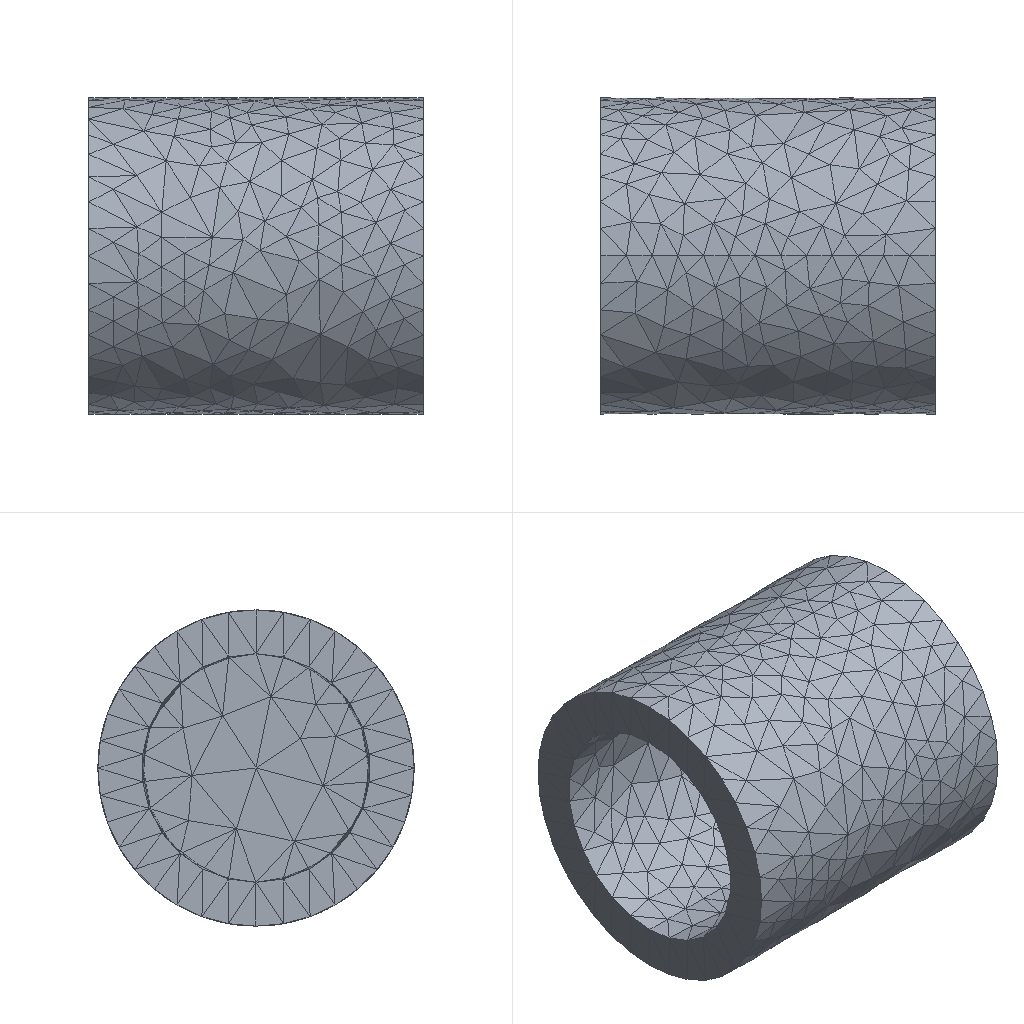Simulation study | ansys workbench
Ansys APDL input file, long lists of numbers shortened:
/batch
/config,noeldb,1     ! force off writing results to database
*get,_wallstrt,active,,time,wall
! ANSYS input file written by Workbench version 2022 R1
! File used for geometry attach:
/title,wbnew--____ (A5)
! ****** Begin Custom Load Command Snippet ******
/COM, ACT Extensions:
/COM,     LSDYNA, 2021.1
/COM,
! ****** End   Custom Load Command Snippet ******
*DIM,_wb_ProjectScratch_dir,string,248
_wb_ProjectScratch_dir(1) = ''
*DIM,_wb_SolverFiles_dir,string,248
_wb_SolverFiles_dir(1) = ''
*DIM,_wb_userfiles_dir,string,248
_wb_userfiles_dir(1) = ''
/com,--- Data in consistent NMM units. See Solving Units in the help system for more information.
/units,MPA
/nopr
/wb,file,start              !  signify a WB generated input file
/prep7
! Turn off shape checking because checks already performed inside WB mesher.
! See help system for more information.
SHPP,OFF,,NOWARN
/nolist
etcon,set             ! allow ANSYS to choose best KEYOP's for 180x elements, resets any applicable keyopt to MAPDL defaults
/com,*********** Nodes for the whole assembly ***********
nblock,3,,5894
(1i9,3e20.9e3)
        1     1.304000000E+03     0.000000000E+00     1.443258926E+02
! (5358 more lines like these left out)
-1
/wb,elem,start            !  set before creation of elements
/com,*********** Elements for Body 1 "__1-FreeParts|__-__1" ***********
et,1,187
eblock,19,solid,,2968
(19i9)
        1        1        1        1        0        0        0        0       10        0        1      310      463      855      443     2861     3860     2866     2860
! (5935 more lines like these left out)
-1
/wb,elem,end               !  done creating elements
/com,*********** Send User Defined Coordinate System(s) ***********
csys,0
toffst,273.15,  ! Temperature offset from absolute zero
/com,*********** Set Reference Temperature ***********
tref,22.
/wb,mat,start              !  starting to send materials
/com,*********** Send Materials ***********
Temperature = 'TEMP' ! Temperature
MP,DENS,1,7.85e-09,	! tonne mm^-3
MP,ALPX,1,1.2e-05,	! C^-1
MP,C,1,434000000,	! mm^2 s^-2 C^-1
MP,KXX,1,60.5,	! tonne mm s^-3 C^-1
MP,RSVX,1,0.00017,	! ohm mm
MP,EX,1,200000,	! tonne s^-2 mm^-1
MP,NUXY,1,0.3,
MP,MURX,1,10000,
/wb,mat,end                !  done sending materials
!************************* Model Summary ********************
!__1-FreeParts|__-__1,	结构钢,	matid,	1
!************************* End Model Summary ********************
! get the diagonal of the bounding box. Needed later for other things
*get,_xmin,node,,mnloc,x
*get,_ymin,node,,mnloc,y
*get,_zmin,node,,mnloc,z
*get,_xmax,node,,mxloc,x
*get,_ymax,node,,mxloc,y
*get,_zmax,node,,mxloc,z
_ASMDIAG=(_xmax-_xmin)*(_xmax-_xmin)+(_ymax-_ymin)*(_ymax-_ymin)+(_zmax-_zmin)*(_zmax-_zmin)
_ASMDIAG=SQRT(_ASMDIAG)
/wb,contact,start          !  starting to send contact
/wb,contact,end            !  done creating contacts
/golist
/wb,load,start             !  starting to send loads
/com,*********** Fixed Supports ***********
CMBLOCK,_FIXEDSU,NODE,      201
(8i10)
         1         2         3         4         5         6         7         8
! (25 more lines like these left out)
cmsel,s,_FIXEDSU
d,all,all
nsel,all
/com,*********** Define Pressure Using Surface Effect Elements "__" ***********
et,2,154
eblock,10,,,762
(15i9)
     4333        2        2        2        0       21        2      152      152      861      862      152      969
! (761 more lines like these left out)
-1
esel,s,type,,2
keyop,2,7,0                ! Use deformed area for application of load
esel,all
/com,*********** Define Pressure Using Surface Effect Elements "__ 2" ***********
et,3,154
eblock,10,,,410
(15i9)
     5095        3        3        3        0       97       98      439      439     1564     1576      439     1568
! (409 more lines like these left out)
-1
esel,s,type,,3
keyop,3,7,0                ! Use deformed area for application of load
esel,all
esel,all
/gst,on,on
fini
*get,_numnode,node,0,count
*get,_numelem,elem,0,count
*get, _MAXELEMNUM, elem, 0, NUM, MAX
*get, _MAXNODENUM, node, 0, NUM, MAX
*get, _MAXELEMTYPE, etyp, 0, NUM, MAX
*get, _MAXREALCONST, real, 0, NUM, MAX
/go
/wb,load,end               !  done creating loads
/com,--- Number of total nodes = %_numnode%
/com,--- Number of contact elements = 1172
/com,--- Number of spring elements = 0
/com,--- Number of bearing elements = 0
/com,--- Number of solid elements = 2968
/com,--- Number of condensed parts = 0
/com,--- Number of total elements = %_numelem%
*get,_wallbsol,active,,time,wall
/com,****************************************************************************
/com,*************************    SOLUTION       ********************************
/com,****************************************************************************
/solu
antype,0                   ! static analysis
_thickRatio=  0     ! Ratio of thick parts in the model
eqsl,sparse,,,,,1
cntr,print,1               ! print out contact info and also make no initial contact an error
dmpoption,emat,no             ! Don't combine emat file for DANSYS
dmpoption,esav,no             ! Don't combine esav file for DANSYS
nldiag,cont,iter           ! print out contact info each equilibrium iteration
rescontrol,,none                 ! Do not keep any restart files
/com,****************************************************
/com,******************* SOLVE FOR LS 1 OF 1 ****************
esel,s,type,,2
nsle
sf,all,pres,20.
esel,s,type,,3
nsle
sf,all,pres,60.
nsel,all
esel,all
esel,all
/nopr
/gopr
nsub,1,1,1
time,1.
outres,erase
outres,all,none
outres,nsol,all,
outres,rsol,all
outres,eangl,all
outres,etmp,all
outres,veng,all
outres,strs,all,
outres,epel,all,
outres,eppl,all,
outres,cont,all,
! *********** WB SOLVE COMMAND ***********
! check interactive state
*get,ANSINTER_,active,,int
*if,ANSINTER_,ne,0,then
/eof
*endif
solve
/com *************** Write FE CONNECTORS *********
CEWRITE,file,ce,,INTE
/com,****************************************************
/com,*************** FINISHED SOLVE FOR LS 1 *************
*get,_wallasol,active,,time,wall
/nopr
*get,_numnode,node,0,count
*get,_numelem,elem,0,count
*get, _MAXELEMNUM, elem, 0, NUM, MAX
*get, _MAXNODENUM, node, 0, NUM, MAX,,,INTERNAL
*get, _MAXELEMTYPE, etyp, 0, NUM, MAX
*get, _MAXREALCONST, real, 0, NUM, MAX
/gopr
/post1
xmlo,ENCODING,ISO-8859-1
xmlo,parm
/xml,parm,xml
fini
/gopr
*get,_walldone,active,,time,wall
_preptime=(_wallbsol-_wallstrt)*3600
_solvtime=(_wallasol-_wallbsol)*3600
_posttime=(_walldone-_wallasol)*3600
_totaltim=(_walldone-_wallstrt)*3600
*get,_dlbratio,active,0,solu,dlbr
*get,_combtime,active,0,solu,comb
*get,_ssmode,active,0,solu,ssmm
*get,_ndofs,active,0,solu,ndof
*get,_sol_end_time,active,0,set,time
*if,_sol_end_time,eq,1.,then
/fclean				!clean distributed files
*endif
/com,--- Total number of nodes = %_numnode%
/com,--- Total number of elements = %_numelem%
/com,--- Element load balance ratio = %_dlbratio%
/com,--- Time to combine distributed files = %_combtime%
/com,--- Sparse memory mode = %_ssmode%
/com,--- Number of DOF = %_ndofs%
/wb,file,end               ! done with WB generated input